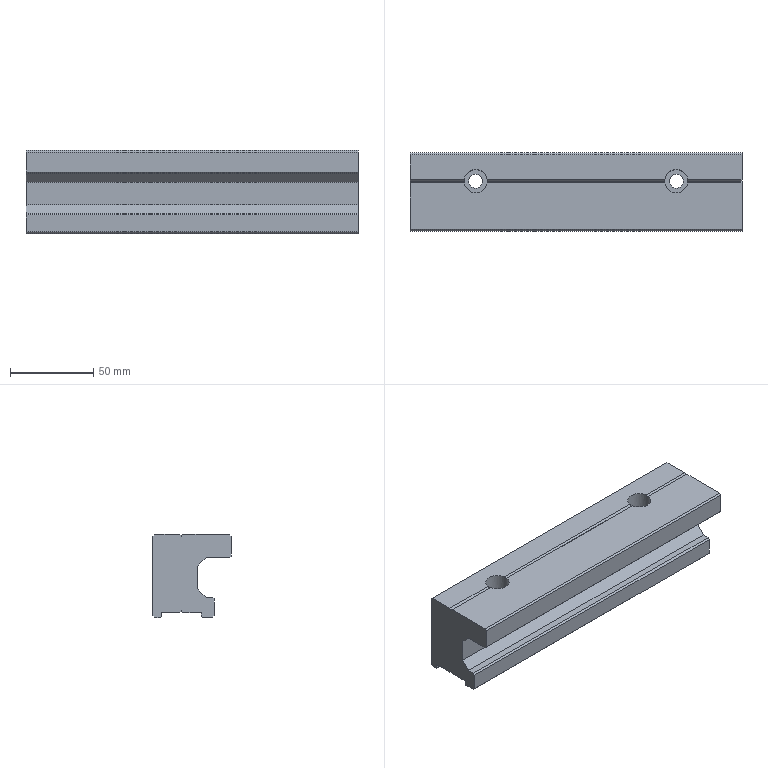Part | NX | features EXTRUDE 3, DATUM_CSYS 2, SKETCH 1 | 1 solid | 44 faces | box 200 x 47 x 50 mm | volume 331921 mm3 | plane 40 | cylinder 4 | commonest cylinder face diameters 8.5 x2 14 x2
STEP:
#1=CARTESIAN_POINT('',(5499.076,6787.516,0.));
#2=VERTEX_POINT('',#1);
#3=CARTESIAN_POINT('',(5485.22,6787.516,0.));
#4=VERTEX_POINT('',#3);
#5=CARTESIAN_POINT('',(5492.148,6786.516,0.));
#6=DIRECTION('',(0.,0.,1.));
#7=DIRECTION('',(1.,0.,0.));
#8=AXIS2_PLACEMENT_3D('',#5,#6,#7);
#9=CIRCLE('',#8,7.);
#10=EDGE_CURVE('',#2,#4,#9,.T.);
#11=ORIENTED_EDGE('',*,*,#10,.F.);
#12=CARTESIAN_POINT('',(5531.718,6787.516,0.));
#13=VERTEX_POINT('',#12);
#14=CARTESIAN_POINT('',(5331.718,6787.516,0.));
#15=DIRECTION('',(1.,0.,0.));
#16=VECTOR('',#15,1000.);
#17=LINE('',#14,#16);
#18=EDGE_CURVE('',#2,#13,#17,.T.);
#19=ORIENTED_EDGE('',*,*,#18,.T.);
#20=CARTESIAN_POINT('',(5531.718,6802.516,0.));
#21=VERTEX_POINT('',#20);
#22=CARTESIAN_POINT('',(5531.718,6787.516,0.));
#23=DIRECTION('',(0.,1.,0.));
#24=VECTOR('',#23,1000.);
#25=LINE('',#22,#24);
#26=EDGE_CURVE('',#13,#21,#25,.T.);
#27=ORIENTED_EDGE('',*,*,#26,.T.);
#28=CARTESIAN_POINT('',(5331.718,6802.516,0.));
#29=VERTEX_POINT('',#28);
#30=CARTESIAN_POINT('',(5331.718,6802.516,0.));
#31=DIRECTION('',(1.,0.,0.));
#32=VECTOR('',#31,1000.);
#33=LINE('',#30,#32);
#34=EDGE_CURVE('',#29,#21,#33,.T.);
#35=ORIENTED_EDGE('',*,*,#34,.F.);
#36=CARTESIAN_POINT('',(5331.718,6787.516,0.));
#37=VERTEX_POINT('',#36);
#38=CARTESIAN_POINT('',(5331.718,6787.516,0.));
#39=DIRECTION('',(0.,1.,0.));
#40=VECTOR('',#39,1000.);
#41=LINE('',#38,#40);
#42=EDGE_CURVE('',#37,#29,#41,.T.);
#43=ORIENTED_EDGE('',*,*,#42,.F.);
#44=CARTESIAN_POINT('',(5364.361,6787.516,0.));
#45=VERTEX_POINT('',#44);
#46=CARTESIAN_POINT('',(5331.718,6787.516,0.));
#47=DIRECTION('',(1.,0.,0.));
#48=VECTOR('',#47,1000.);
#49=LINE('',#46,#48);
#50=EDGE_CURVE('',#37,#45,#49,.T.);
#51=ORIENTED_EDGE('',*,*,#50,.T.);
#52=CARTESIAN_POINT('',(5378.217,6787.516,0.));
#53=VERTEX_POINT('',#52);
#54=CARTESIAN_POINT('',(5371.289,6786.516,0.));
#55=DIRECTION('',(0.,0.,1.));
#56=DIRECTION('',(1.,0.,0.));
#57=AXIS2_PLACEMENT_3D('',#54,#55,#56);
#58=CIRCLE('',#57,7.);
#59=EDGE_CURVE('',#53,#45,#58,.T.);
#60=ORIENTED_EDGE('',*,*,#59,.F.);
#61=CARTESIAN_POINT('',(5331.718,6787.516,0.));
#62=DIRECTION('',(1.,0.,0.));
#63=VECTOR('',#62,1000.);
#64=LINE('',#61,#63);
#65=EDGE_CURVE('',#53,#4,#64,.T.);
#66=ORIENTED_EDGE('',*,*,#65,.T.);
#67=EDGE_LOOP('',(#11,#19,#27,#35,#43,#51,#60,#66));
#68=FACE_BOUND('',#67,.T.);
#69=CARTESIAN_POINT('',(5331.718,6787.516,0.));
#70=DIRECTION('',(0.,0.,-1.));
#71=DIRECTION('',(-1.,0.,0.));
#72=AXIS2_PLACEMENT_3D('',#69,#70,#71);
#73=PLANE('',#72);
#74=ADVANCED_FACE('',(#68),#73,.F.);
#75=CARTESIAN_POINT('',(5485.22,6785.516,0.));
#76=VERTEX_POINT('',#75);
#77=CARTESIAN_POINT('',(5499.076,6785.516,0.));
#78=VERTEX_POINT('',#77);
#79=CARTESIAN_POINT('',(5492.148,6786.516,0.));
#80=DIRECTION('',(0.,0.,1.));
#81=DIRECTION('',(1.,0.,0.));
#82=AXIS2_PLACEMENT_3D('',#79,#80,#81);
#83=CIRCLE('',#82,7.);
#84=EDGE_CURVE('',#76,#78,#83,.T.);
#85=ORIENTED_EDGE('',*,*,#84,.F.);
#86=CARTESIAN_POINT('',(5378.217,6785.516,0.));
#87=VERTEX_POINT('',#86);
#88=CARTESIAN_POINT('',(5331.718,6785.516,0.));
#89=DIRECTION('',(1.,0.,0.));
#90=VECTOR('',#89,1000.);
#91=LINE('',#88,#90);
#92=EDGE_CURVE('',#87,#76,#91,.T.);
#93=ORIENTED_EDGE('',*,*,#92,.F.);
#94=CARTESIAN_POINT('',(5364.361,6785.516,0.));
#95=VERTEX_POINT('',#94);
#96=CARTESIAN_POINT('',(5371.289,6786.516,0.));
#97=DIRECTION('',(0.,0.,1.));
#98=DIRECTION('',(1.,0.,0.));
#99=AXIS2_PLACEMENT_3D('',#96,#97,#98);
#100=CIRCLE('',#99,7.);
#101=EDGE_CURVE('',#95,#87,#100,.T.);
#102=ORIENTED_EDGE('',*,*,#101,.F.);
#103=CARTESIAN_POINT('',(5331.718,6785.516,0.));
#104=VERTEX_POINT('',#103);
#105=CARTESIAN_POINT('',(5331.718,6785.516,0.));
#106=DIRECTION('',(1.,0.,0.));
#107=VECTOR('',#106,1000.);
#108=LINE('',#105,#107);
#109=EDGE_CURVE('',#104,#95,#108,.T.);
#110=ORIENTED_EDGE('',*,*,#109,.F.);
#111=CARTESIAN_POINT('',(5331.718,6757.516,0.));
#112=VERTEX_POINT('',#111);
#113=CARTESIAN_POINT('',(5331.718,6757.516,0.));
#114=DIRECTION('',(0.,1.,0.));
#115=VECTOR('',#114,1000.);
#116=LINE('',#113,#115);
#117=EDGE_CURVE('',#112,#104,#116,.T.);
#118=ORIENTED_EDGE('',*,*,#117,.F.);
#119=CARTESIAN_POINT('',(5531.718,6757.516,0.));
#120=VERTEX_POINT('',#119);
#121=CARTESIAN_POINT('',(5331.718,6757.516,0.));
#122=DIRECTION('',(1.,0.,0.));
#123=VECTOR('',#122,1000.);
#124=LINE('',#121,#123);
#125=EDGE_CURVE('',#112,#120,#124,.T.);
#126=ORIENTED_EDGE('',*,*,#125,.T.);
#127=CARTESIAN_POINT('',(5531.718,6785.516,0.));
#128=VERTEX_POINT('',#127);
#129=CARTESIAN_POINT('',(5531.718,6757.516,0.));
#130=DIRECTION('',(0.,1.,0.));
#131=VECTOR('',#130,1000.);
#132=LINE('',#129,#131);
#133=EDGE_CURVE('',#120,#128,#132,.T.);
#134=ORIENTED_EDGE('',*,*,#133,.T.);
#135=CARTESIAN_POINT('',(5331.718,6785.516,0.));
#136=DIRECTION('',(1.,0.,0.));
#137=VECTOR('',#136,1000.);
#138=LINE('',#135,#137);
#139=EDGE_CURVE('',#78,#128,#138,.T.);
#140=ORIENTED_EDGE('',*,*,#139,.F.);
#141=EDGE_LOOP('',(#85,#93,#102,#110,#118,#126,#134,#140));
#142=FACE_BOUND('',#141,.T.);
#143=CARTESIAN_POINT('',(5331.718,6757.516,0.));
#144=DIRECTION('',(0.,0.,-1.));
#145=DIRECTION('',(-1.,0.,0.));
#146=AXIS2_PLACEMENT_3D('',#143,#144,#145);
#147=PLANE('',#146);
#148=ADVANCED_FACE('',(#142),#147,.F.);
#149=CARTESIAN_POINT('',(5375.419,6785.516,-47.));
#150=VERTEX_POINT('',#149);
#151=CARTESIAN_POINT('',(5367.158,6785.516,-47.));
#152=VERTEX_POINT('',#151);
#153=CARTESIAN_POINT('',(5371.289,6786.516,-47.));
#154=DIRECTION('',(0.,0.,1.));
#155=DIRECTION('',(1.,0.,0.));
#156=AXIS2_PLACEMENT_3D('',#153,#154,#155);
#157=CIRCLE('',#156,4.25);
#158=EDGE_CURVE('',#150,#152,#157,.F.);
#159=ORIENTED_EDGE('',*,*,#158,.T.);
#160=CARTESIAN_POINT('',(5367.039,6786.516,-46.));
#161=VERTEX_POINT('',#160);
#162=CARTESIAN_POINT('',(5371.289,6786.516,-46.));
#163=DIRECTION('',(0.,-0.7071,0.7071));
#164=DIRECTION('',(0.,0.7071,0.7071));
#165=AXIS2_PLACEMENT_3D('',#162,#163,#164);
#166=ELLIPSE('',#165,6.01,4.25);
#167=EDGE_CURVE('',#152,#161,#166,.F.);
#168=ORIENTED_EDGE('',*,*,#167,.T.);
#169=CARTESIAN_POINT('',(5367.158,6787.516,-47.));
#170=VERTEX_POINT('',#169);
#171=CARTESIAN_POINT('',(5371.289,6786.516,-46.));
#172=DIRECTION('',(0.,0.7071,0.7071));
#173=DIRECTION('',(0.,-0.7071,0.7071));
#174=AXIS2_PLACEMENT_3D('',#171,#172,#173);
#175=ELLIPSE('',#174,6.01,4.25);
#176=EDGE_CURVE('',#161,#170,#175,.F.);
#177=ORIENTED_EDGE('',*,*,#176,.T.);
#178=CARTESIAN_POINT('',(5375.419,6787.516,-47.));
#179=VERTEX_POINT('',#178);
#180=CARTESIAN_POINT('',(5371.289,6786.516,-47.));
#181=DIRECTION('',(0.,0.,1.));
#182=DIRECTION('',(1.,0.,0.));
#183=AXIS2_PLACEMENT_3D('',#180,#181,#182);
#184=CIRCLE('',#183,4.25);
#185=EDGE_CURVE('',#170,#179,#184,.F.);
#186=ORIENTED_EDGE('',*,*,#185,.T.);
#187=CARTESIAN_POINT('',(5375.539,6786.516,-46.));
#188=VERTEX_POINT('',#187);
#189=CARTESIAN_POINT('',(5371.289,6786.516,-46.));
#190=DIRECTION('',(0.,0.7071,0.7071));
#191=DIRECTION('',(0.,-0.7071,0.7071));
#192=AXIS2_PLACEMENT_3D('',#189,#190,#191);
#193=ELLIPSE('',#192,6.01,4.25);
#194=EDGE_CURVE('',#179,#188,#193,.F.);
#195=ORIENTED_EDGE('',*,*,#194,.T.);
#196=CARTESIAN_POINT('',(5371.289,6786.516,-46.));
#197=DIRECTION('',(0.,-0.7071,0.7071));
#198=DIRECTION('',(0.,0.7071,0.7071));
#199=AXIS2_PLACEMENT_3D('',#196,#197,#198);
#200=ELLIPSE('',#199,6.01,4.25);
#201=EDGE_CURVE('',#188,#150,#200,.F.);
#202=ORIENTED_EDGE('',*,*,#201,.T.);
#203=EDGE_LOOP('',(#159,#168,#177,#186,#195,#202));
#204=FACE_BOUND('',#203,.T.);
#205=CARTESIAN_POINT('',(5375.539,6786.516,-12.));
#206=VERTEX_POINT('',#205);
#207=CARTESIAN_POINT('',(5371.289,6786.516,-12.));
#208=DIRECTION('',(0.,0.,1.));
#209=DIRECTION('',(1.,0.,0.));
#210=AXIS2_PLACEMENT_3D('',#207,#208,#209);
#211=CIRCLE('',#210,4.25);
#212=EDGE_CURVE('',#206,#206,#211,.F.);
#213=ORIENTED_EDGE('',*,*,#212,.F.);
#214=EDGE_LOOP('',(#213));
#215=FACE_BOUND('',#214,.T.);
#216=CARTESIAN_POINT('',(5371.289,6786.516,-55000.));
#217=DIRECTION('',(0.,0.,1.));
#218=DIRECTION('',(1.,0.,0.));
#219=AXIS2_PLACEMENT_3D('',#216,#217,#218);
#220=CYLINDRICAL_SURFACE('',#219,4.25);
#221=ADVANCED_FACE('',(#204,#215),#220,.F.);
#222=CARTESIAN_POINT('',(5496.279,6785.516,-47.));
#223=VERTEX_POINT('',#222);
#224=CARTESIAN_POINT('',(5488.017,6785.516,-47.));
#225=VERTEX_POINT('',#224);
#226=CARTESIAN_POINT('',(5492.148,6786.516,-47.));
#227=DIRECTION('',(0.,0.,1.));
#228=DIRECTION('',(1.,0.,0.));
#229=AXIS2_PLACEMENT_3D('',#226,#227,#228);
#230=CIRCLE('',#229,4.25);
#231=EDGE_CURVE('',#223,#225,#230,.F.);
#232=ORIENTED_EDGE('',*,*,#231,.T.);
#233=CARTESIAN_POINT('',(5487.898,6786.516,-46.));
#234=VERTEX_POINT('',#233);
#235=CARTESIAN_POINT('',(5492.148,6786.516,-46.));
#236=DIRECTION('',(0.,-0.7071,0.7071));
#237=DIRECTION('',(0.,0.7071,0.7071));
#238=AXIS2_PLACEMENT_3D('',#235,#236,#237);
#239=ELLIPSE('',#238,6.01,4.25);
#240=EDGE_CURVE('',#225,#234,#239,.F.);
#241=ORIENTED_EDGE('',*,*,#240,.T.);
#242=CARTESIAN_POINT('',(5488.017,6787.516,-47.));
#243=VERTEX_POINT('',#242);
#244=CARTESIAN_POINT('',(5492.148,6786.516,-46.));
#245=DIRECTION('',(0.,0.7071,0.7071));
#246=DIRECTION('',(0.,-0.7071,0.7071));
#247=AXIS2_PLACEMENT_3D('',#244,#245,#246);
#248=ELLIPSE('',#247,6.01,4.25);
#249=EDGE_CURVE('',#234,#243,#248,.F.);
#250=ORIENTED_EDGE('',*,*,#249,.T.);
#251=CARTESIAN_POINT('',(5496.279,6787.516,-47.));
#252=VERTEX_POINT('',#251);
#253=CARTESIAN_POINT('',(5492.148,6786.516,-47.));
#254=DIRECTION('',(0.,0.,1.));
#255=DIRECTION('',(1.,0.,0.));
#256=AXIS2_PLACEMENT_3D('',#253,#254,#255);
#257=CIRCLE('',#256,4.25);
#258=EDGE_CURVE('',#243,#252,#257,.F.);
#259=ORIENTED_EDGE('',*,*,#258,.T.);
#260=CARTESIAN_POINT('',(5496.398,6786.516,-46.));
#261=VERTEX_POINT('',#260);
#262=CARTESIAN_POINT('',(5492.148,6786.516,-46.));
#263=DIRECTION('',(0.,0.7071,0.7071));
#264=DIRECTION('',(0.,-0.7071,0.7071));
#265=AXIS2_PLACEMENT_3D('',#262,#263,#264);
#266=ELLIPSE('',#265,6.01,4.25);
#267=EDGE_CURVE('',#252,#261,#266,.F.);
#268=ORIENTED_EDGE('',*,*,#267,.T.);
#269=CARTESIAN_POINT('',(5492.148,6786.516,-46.));
#270=DIRECTION('',(0.,-0.7071,0.7071));
#271=DIRECTION('',(0.,0.7071,0.7071));
#272=AXIS2_PLACEMENT_3D('',#269,#270,#271);
#273=ELLIPSE('',#272,6.01,4.25);
#274=EDGE_CURVE('',#261,#223,#273,.F.);
#275=ORIENTED_EDGE('',*,*,#274,.T.);
#276=EDGE_LOOP('',(#232,#241,#250,#259,#268,#275));
#277=FACE_BOUND('',#276,.T.);
#278=CARTESIAN_POINT('',(5496.398,6786.516,-12.));
#279=VERTEX_POINT('',#278);
#280=CARTESIAN_POINT('',(5492.148,6786.516,-12.));
#281=DIRECTION('',(0.,0.,1.));
#282=DIRECTION('',(1.,0.,0.));
#283=AXIS2_PLACEMENT_3D('',#280,#281,#282);
#284=CIRCLE('',#283,4.25);
#285=EDGE_CURVE('',#279,#279,#284,.F.);
#286=ORIENTED_EDGE('',*,*,#285,.F.);
#287=EDGE_LOOP('',(#286));
#288=FACE_BOUND('',#287,.T.);
#289=CARTESIAN_POINT('',(5492.148,6786.516,-55000.));
#290=DIRECTION('',(0.,0.,1.));
#291=DIRECTION('',(1.,0.,0.));
#292=AXIS2_PLACEMENT_3D('',#289,#290,#291);
#293=CYLINDRICAL_SURFACE('',#292,4.25);
#294=ADVANCED_FACE('',(#277,#288),#293,.F.);
#295=ORIENTED_EDGE('',*,*,#258,.F.);
#296=CARTESIAN_POINT('',(5331.718,6787.516,-47.));
#297=DIRECTION('',(1.,0.,0.));
#298=VECTOR('',#297,1000.);
#299=LINE('',#296,#298);
#300=EDGE_CURVE('',#179,#243,#299,.T.);
#301=ORIENTED_EDGE('',*,*,#300,.F.);
#302=ORIENTED_EDGE('',*,*,#185,.F.);
#303=CARTESIAN_POINT('',(5331.718,6787.516,-47.));
#304=VERTEX_POINT('',#303);
#305=CARTESIAN_POINT('',(5331.718,6787.516,-47.));
#306=DIRECTION('',(1.,0.,0.));
#307=VECTOR('',#306,1000.);
#308=LINE('',#305,#307);
#309=EDGE_CURVE('',#304,#170,#308,.T.);
#310=ORIENTED_EDGE('',*,*,#309,.F.);
#311=CARTESIAN_POINT('',(5331.718,6798.591,-47.));
#312=VERTEX_POINT('',#311);
#313=CARTESIAN_POINT('',(5331.718,6798.591,-47.));
#314=DIRECTION('',(0.,-1.,0.));
#315=VECTOR('',#314,1000.);
#316=LINE('',#313,#315);
#317=EDGE_CURVE('',#312,#304,#316,.T.);
#318=ORIENTED_EDGE('',*,*,#317,.F.);
#319=CARTESIAN_POINT('',(5531.718,6798.591,-47.));
#320=VERTEX_POINT('',#319);
#321=CARTESIAN_POINT('',(5331.718,6798.591,-47.));
#322=DIRECTION('',(1.,0.,0.));
#323=VECTOR('',#322,1000.);
#324=LINE('',#321,#323);
#325=EDGE_CURVE('',#312,#320,#324,.T.);
#326=ORIENTED_EDGE('',*,*,#325,.T.);
#327=CARTESIAN_POINT('',(5531.718,6787.516,-47.));
#328=VERTEX_POINT('',#327);
#329=CARTESIAN_POINT('',(5531.718,6798.591,-47.));
#330=DIRECTION('',(0.,-1.,0.));
#331=VECTOR('',#330,1000.);
#332=LINE('',#329,#331);
#333=EDGE_CURVE('',#320,#328,#332,.T.);
#334=ORIENTED_EDGE('',*,*,#333,.T.);
#335=CARTESIAN_POINT('',(5331.718,6787.516,-47.));
#336=DIRECTION('',(1.,0.,0.));
#337=VECTOR('',#336,1000.);
#338=LINE('',#335,#337);
#339=EDGE_CURVE('',#252,#328,#338,.T.);
#340=ORIENTED_EDGE('',*,*,#339,.F.);
#341=EDGE_LOOP('',(#295,#301,#302,#310,#318,#326,#334,#340));
#342=FACE_BOUND('',#341,.T.);
#343=CARTESIAN_POINT('',(5331.718,6798.591,-47.));
#344=DIRECTION('',(0.,0.,1.));
#345=DIRECTION('',(1.,0.,0.));
#346=AXIS2_PLACEMENT_3D('',#343,#344,#345);
#347=PLANE('',#346);
#348=ADVANCED_FACE('',(#342),#347,.F.);
#349=ORIENTED_EDGE('',*,*,#249,.F.);
#350=CARTESIAN_POINT('',(5331.718,6786.516,-46.));
#351=DIRECTION('',(1.,0.,0.));
#352=VECTOR('',#351,1000.);
#353=LINE('',#350,#352);
#354=EDGE_CURVE('',#188,#234,#353,.T.);
#355=ORIENTED_EDGE('',*,*,#354,.F.);
#356=ORIENTED_EDGE('',*,*,#194,.F.);
#357=ORIENTED_EDGE('',*,*,#300,.T.);
#358=EDGE_LOOP('',(#349,#355,#356,#357));
#359=FACE_BOUND('',#358,.T.);
#360=CARTESIAN_POINT('',(5331.718,6787.516,-47.));
#361=DIRECTION('',(0.,0.7071,0.7071));
#362=DIRECTION('',(0.,-0.7071,0.7071));
#363=AXIS2_PLACEMENT_3D('',#360,#361,#362);
#364=PLANE('',#363);
#365=ADVANCED_FACE('',(#359),#364,.F.);
#366=ORIENTED_EDGE('',*,*,#267,.F.);
#367=ORIENTED_EDGE('',*,*,#339,.T.);
#368=CARTESIAN_POINT('',(5531.718,6786.516,-46.));
#369=VERTEX_POINT('',#368);
#370=CARTESIAN_POINT('',(5531.718,6787.516,-47.));
#371=DIRECTION('',(0.,-0.7071,0.7071));
#372=VECTOR('',#371,1000.);
#373=LINE('',#370,#372);
#374=EDGE_CURVE('',#328,#369,#373,.T.);
#375=ORIENTED_EDGE('',*,*,#374,.T.);
#376=CARTESIAN_POINT('',(5331.718,6786.516,-46.));
#377=DIRECTION('',(1.,0.,0.));
#378=VECTOR('',#377,1000.);
#379=LINE('',#376,#378);
#380=EDGE_CURVE('',#261,#369,#379,.T.);
#381=ORIENTED_EDGE('',*,*,#380,.F.);
#382=EDGE_LOOP('',(#366,#367,#375,#381));
#383=FACE_BOUND('',#382,.T.);
#384=CARTESIAN_POINT('',(5331.718,6787.516,-47.));
#385=DIRECTION('',(0.,0.7071,0.7071));
#386=DIRECTION('',(0.,-0.7071,0.7071));
#387=AXIS2_PLACEMENT_3D('',#384,#385,#386);
#388=PLANE('',#387);
#389=ADVANCED_FACE('',(#383),#388,.F.);
#390=ORIENTED_EDGE('',*,*,#176,.F.);
#391=CARTESIAN_POINT('',(5331.718,6786.516,-46.));
#392=VERTEX_POINT('',#391);
#393=CARTESIAN_POINT('',(5331.718,6786.516,-46.));
#394=DIRECTION('',(1.,0.,0.));
#395=VECTOR('',#394,1000.);
#396=LINE('',#393,#395);
#397=EDGE_CURVE('',#392,#161,#396,.T.);
#398=ORIENTED_EDGE('',*,*,#397,.F.);
#399=CARTESIAN_POINT('',(5331.718,6787.516,-47.));
#400=DIRECTION('',(0.,-0.7071,0.7071));
#401=VECTOR('',#400,1000.);
#402=LINE('',#399,#401);
#403=EDGE_CURVE('',#304,#392,#402,.T.);
#404=ORIENTED_EDGE('',*,*,#403,.F.);
#405=ORIENTED_EDGE('',*,*,#309,.T.);
#406=EDGE_LOOP('',(#390,#398,#404,#405));
#407=FACE_BOUND('',#406,.T.);
#408=CARTESIAN_POINT('',(5331.718,6787.516,-47.));
#409=DIRECTION('',(0.,0.7071,0.7071));
#410=DIRECTION('',(0.,-0.7071,0.7071));
#411=AXIS2_PLACEMENT_3D('',#408,#409,#410);
#412=PLANE('',#411);
#413=ADVANCED_FACE('',(#407),#412,.F.);
#414=ORIENTED_EDGE('',*,*,#274,.F.);
#415=ORIENTED_EDGE('',*,*,#380,.T.);
#416=CARTESIAN_POINT('',(5531.718,6785.516,-47.));
#417=VERTEX_POINT('',#416);
#418=CARTESIAN_POINT('',(5531.718,6786.516,-46.));
#419=DIRECTION('',(0.,-0.7071,-0.7071));
#420=VECTOR('',#419,1000.);
#421=LINE('',#418,#420);
#422=EDGE_CURVE('',#369,#417,#421,.T.);
#423=ORIENTED_EDGE('',*,*,#422,.T.);
#424=CARTESIAN_POINT('',(5331.718,6785.516,-47.));
#425=DIRECTION('',(1.,0.,0.));
#426=VECTOR('',#425,1000.);
#427=LINE('',#424,#426);
#428=EDGE_CURVE('',#223,#417,#427,.T.);
#429=ORIENTED_EDGE('',*,*,#428,.F.);
#430=EDGE_LOOP('',(#414,#415,#423,#429));
#431=FACE_BOUND('',#430,.T.);
#432=CARTESIAN_POINT('',(5331.718,6786.516,-46.));
#433=DIRECTION('',(0.,-0.7071,0.7071));
#434=DIRECTION('',(0.,-0.7071,-0.7071));
#435=AXIS2_PLACEMENT_3D('',#432,#433,#434);
#436=PLANE('',#435);
#437=ADVANCED_FACE('',(#431),#436,.F.);
#438=ORIENTED_EDGE('',*,*,#240,.F.);
#439=CARTESIAN_POINT('',(5331.718,6785.516,-47.));
#440=DIRECTION('',(1.,0.,0.));
#441=VECTOR('',#440,1000.);
#442=LINE('',#439,#441);
#443=EDGE_CURVE('',#150,#225,#442,.T.);
#444=ORIENTED_EDGE('',*,*,#443,.F.);
#445=ORIENTED_EDGE('',*,*,#201,.F.);
#446=ORIENTED_EDGE('',*,*,#354,.T.);
#447=EDGE_LOOP('',(#438,#444,#445,#446));
#448=FACE_BOUND('',#447,.T.);
#449=CARTESIAN_POINT('',(5331.718,6786.516,-46.));
#450=DIRECTION('',(0.,-0.7071,0.7071));
#451=DIRECTION('',(0.,-0.7071,-0.7071));
#452=AXIS2_PLACEMENT_3D('',#449,#450,#451);
#453=PLANE('',#452);
#454=ADVANCED_FACE('',(#448),#453,.F.);
#455=ORIENTED_EDGE('',*,*,#167,.F.);
#456=CARTESIAN_POINT('',(5331.718,6785.516,-47.));
#457=VERTEX_POINT('',#456);
#458=CARTESIAN_POINT('',(5331.718,6785.516,-47.));
#459=DIRECTION('',(1.,0.,0.));
#460=VECTOR('',#459,1000.);
#461=LINE('',#458,#460);
#462=EDGE_CURVE('',#457,#152,#461,.T.);
#463=ORIENTED_EDGE('',*,*,#462,.F.);
#464=CARTESIAN_POINT('',(5331.718,6786.516,-46.));
#465=DIRECTION('',(0.,-0.7071,-0.7071));
#466=VECTOR('',#465,1000.);
#467=LINE('',#464,#466);
#468=EDGE_CURVE('',#392,#457,#467,.T.);
#469=ORIENTED_EDGE('',*,*,#468,.F.);
#470=ORIENTED_EDGE('',*,*,#397,.T.);
#471=EDGE_LOOP('',(#455,#463,#469,#470));
#472=FACE_BOUND('',#471,.T.);
#473=CARTESIAN_POINT('',(5331.718,6786.516,-46.));
#474=DIRECTION('',(0.,-0.7071,0.7071));
#475=DIRECTION('',(0.,-0.7071,-0.7071));
#476=AXIS2_PLACEMENT_3D('',#473,#474,#475);
#477=PLANE('',#476);
#478=ADVANCED_FACE('',(#472),#477,.F.);
#479=ORIENTED_EDGE('',*,*,#231,.F.);
#480=ORIENTED_EDGE('',*,*,#428,.T.);
#481=CARTESIAN_POINT('',(5531.718,6774.441,-47.));
#482=VERTEX_POINT('',#481);
#483=CARTESIAN_POINT('',(5531.718,6785.516,-47.));
#484=DIRECTION('',(0.,-1.,0.));
#485=VECTOR('',#484,1000.);
#486=LINE('',#483,#485);
#487=EDGE_CURVE('',#417,#482,#486,.T.);
#488=ORIENTED_EDGE('',*,*,#487,.T.);
#489=CARTESIAN_POINT('',(5331.718,6774.441,-47.));
#490=VERTEX_POINT('',#489);
#491=CARTESIAN_POINT('',(5331.718,6774.441,-47.));
#492=DIRECTION('',(1.,0.,0.));
#493=VECTOR('',#492,1000.);
#494=LINE('',#491,#493);
#495=EDGE_CURVE('',#490,#482,#494,.T.);
#496=ORIENTED_EDGE('',*,*,#495,.F.);
#497=CARTESIAN_POINT('',(5331.718,6785.516,-47.));
#498=DIRECTION('',(0.,-1.,0.));
#499=VECTOR('',#498,1000.);
#500=LINE('',#497,#499);
#501=EDGE_CURVE('',#457,#490,#500,.T.);
#502=ORIENTED_EDGE('',*,*,#501,.F.);
#503=ORIENTED_EDGE('',*,*,#462,.T.);
#504=ORIENTED_EDGE('',*,*,#158,.F.);
#505=ORIENTED_EDGE('',*,*,#443,.T.);
#506=EDGE_LOOP('',(#479,#480,#488,#496,#502,#503,#504,#505));
#507=FACE_BOUND('',#506,.T.);
#508=CARTESIAN_POINT('',(5331.718,6785.516,-47.));
#509=DIRECTION('',(0.,0.,1.));
#510=DIRECTION('',(1.,0.,0.));
#511=AXIS2_PLACEMENT_3D('',#508,#509,#510);
#512=PLANE('',#511);
#513=ADVANCED_FACE('',(#507),#512,.F.);
#514=ORIENTED_EDGE('',*,*,#92,.T.);
#515=CARTESIAN_POINT('',(5485.148,6786.516,-1.));
#516=VERTEX_POINT('',#515);
#517=CARTESIAN_POINT('',(5492.148,6786.516,-1.));
#518=DIRECTION('',(0.,-0.7071,-0.7071));
#519=DIRECTION('',(0.,-0.7071,0.7071));
#520=AXIS2_PLACEMENT_3D('',#517,#518,#519);
#521=ELLIPSE('',#520,9.899,7.);
#522=EDGE_CURVE('',#76,#516,#521,.T.);
#523=ORIENTED_EDGE('',*,*,#522,.T.);
#524=CARTESIAN_POINT('',(5378.289,6786.516,-1.));
#525=VERTEX_POINT('',#524);
#526=CARTESIAN_POINT('',(5331.718,6786.516,-1.));
#527=DIRECTION('',(1.,0.,0.));
#528=VECTOR('',#527,1000.);
#529=LINE('',#526,#528);
#530=EDGE_CURVE('',#525,#516,#529,.T.);
#531=ORIENTED_EDGE('',*,*,#530,.F.);
#532=CARTESIAN_POINT('',(5371.289,6786.516,-1.));
#533=DIRECTION('',(0.,-0.7071,-0.7071));
#534=DIRECTION('',(0.,-0.7071,0.7071));
#535=AXIS2_PLACEMENT_3D('',#532,#533,#534);
#536=ELLIPSE('',#535,9.899,7.);
#537=EDGE_CURVE('',#525,#87,#536,.T.);
#538=ORIENTED_EDGE('',*,*,#537,.T.);
#539=EDGE_LOOP('',(#514,#523,#531,#538));
#540=FACE_BOUND('',#539,.T.);
#541=CARTESIAN_POINT('',(5331.718,6785.516,0.));
#542=DIRECTION('',(0.,-0.7071,-0.7071));
#543=DIRECTION('',(0.,0.7071,-0.7071));
#544=AXIS2_PLACEMENT_3D('',#541,#542,#543);
#545=PLANE('',#544);
#546=ADVANCED_FACE('',(#540),#545,.F.);
#547=ORIENTED_EDGE('',*,*,#109,.T.);
#548=CARTESIAN_POINT('',(5364.289,6786.516,-1.));
#549=VERTEX_POINT('',#548);
#550=CARTESIAN_POINT('',(5371.289,6786.516,-1.));
#551=DIRECTION('',(0.,-0.7071,-0.7071));
#552=DIRECTION('',(0.,-0.7071,0.7071));
#553=AXIS2_PLACEMENT_3D('',#550,#551,#552);
#554=ELLIPSE('',#553,9.899,7.);
#555=EDGE_CURVE('',#95,#549,#554,.T.);
#556=ORIENTED_EDGE('',*,*,#555,.T.);
#557=CARTESIAN_POINT('',(5331.718,6786.516,-1.));
#558=VERTEX_POINT('',#557);
#559=CARTESIAN_POINT('',(5331.718,6786.516,-1.));
#560=DIRECTION('',(1.,0.,0.));
#561=VECTOR('',#560,1000.);
#562=LINE('',#559,#561);
#563=EDGE_CURVE('',#558,#549,#562,.T.);
#564=ORIENTED_EDGE('',*,*,#563,.F.);
#565=CARTESIAN_POINT('',(5331.718,6785.516,0.));
#566=DIRECTION('',(0.,0.7071,-0.7071));
#567=VECTOR('',#566,1000.);
#568=LINE('',#565,#567);
#569=EDGE_CURVE('',#104,#558,#568,.T.);
#570=ORIENTED_EDGE('',*,*,#569,.F.);
#571=EDGE_LOOP('',(#547,#556,#564,#570));
#572=FACE_BOUND('',#571,.T.);
#573=CARTESIAN_POINT('',(5331.718,6785.516,0.));
#574=DIRECTION('',(0.,-0.7071,-0.7071));
#575=DIRECTION('',(0.,0.7071,-0.7071));
#576=AXIS2_PLACEMENT_3D('',#573,#574,#575);
#577=PLANE('',#576);
#578=ADVANCED_FACE('',(#572),#577,.F.);
#579=ORIENTED_EDGE('',*,*,#18,.F.);
#580=CARTESIAN_POINT('',(5499.148,6786.516,-1.));
#581=VERTEX_POINT('',#580);
#582=CARTESIAN_POINT('',(5492.148,6786.516,-1.));
#583=DIRECTION('',(0.,0.7071,-0.7071));
#584=DIRECTION('',(0.,0.7071,0.7071));
#585=AXIS2_PLACEMENT_3D('',#582,#583,#584);
#586=ELLIPSE('',#585,9.899,7.);
#587=EDGE_CURVE('',#2,#581,#586,.T.);
#588=ORIENTED_EDGE('',*,*,#587,.T.);
#589=CARTESIAN_POINT('',(5531.718,6786.516,-1.));
#590=VERTEX_POINT('',#589);
#591=CARTESIAN_POINT('',(5331.718,6786.516,-1.));
#592=DIRECTION('',(1.,0.,0.));
#593=VECTOR('',#592,1000.);
#594=LINE('',#591,#593);
#595=EDGE_CURVE('',#581,#590,#594,.T.);
#596=ORIENTED_EDGE('',*,*,#595,.T.);
#597=CARTESIAN_POINT('',(5531.718,6786.516,-1.));
#598=DIRECTION('',(0.,0.7071,0.7071));
#599=VECTOR('',#598,1000.);
#600=LINE('',#597,#599);
#601=EDGE_CURVE('',#590,#13,#600,.T.);
#602=ORIENTED_EDGE('',*,*,#601,.T.);
#603=EDGE_LOOP('',(#579,#588,#596,#602));
#604=FACE_BOUND('',#603,.T.);
#605=CARTESIAN_POINT('',(5331.718,6786.516,-1.));
#606=DIRECTION('',(0.,0.7071,-0.7071));
#607=DIRECTION('',(0.,0.7071,0.7071));
#608=AXIS2_PLACEMENT_3D('',#605,#606,#607);
#609=PLANE('',#608);
#610=ADVANCED_FACE('',(#604),#609,.F.);
#611=ORIENTED_EDGE('',*,*,#530,.T.);
#612=CARTESIAN_POINT('',(5492.148,6786.516,-1.));
#613=DIRECTION('',(0.,0.7071,-0.7071));
#614=DIRECTION('',(0.,0.7071,0.7071));
#615=AXIS2_PLACEMENT_3D('',#612,#613,#614);
#616=ELLIPSE('',#615,9.899,7.);
#617=EDGE_CURVE('',#516,#4,#616,.T.);
#618=ORIENTED_EDGE('',*,*,#617,.T.);
#619=ORIENTED_EDGE('',*,*,#65,.F.);
#620=CARTESIAN_POINT('',(5371.289,6786.516,-1.));
#621=DIRECTION('',(0.,0.7071,-0.7071));
#622=DIRECTION('',(0.,0.7071,0.7071));
#623=AXIS2_PLACEMENT_3D('',#620,#621,#622);
#624=ELLIPSE('',#623,9.899,7.);
#625=EDGE_CURVE('',#53,#525,#624,.T.);
#626=ORIENTED_EDGE('',*,*,#625,.T.);
#627=EDGE_LOOP('',(#611,#618,#619,#626));
#628=FACE_BOUND('',#627,.T.);
#629=CARTESIAN_POINT('',(5331.718,6786.516,-1.));
#630=DIRECTION('',(0.,0.7071,-0.7071));
#631=DIRECTION('',(0.,0.7071,0.7071));
#632=AXIS2_PLACEMENT_3D('',#629,#630,#631);
#633=PLANE('',#632);
#634=ADVANCED_FACE('',(#628),#633,.F.);
#635=CARTESIAN_POINT('',(5531.718,6803.516,-1.));
#636=VERTEX_POINT('',#635);
#637=CARTESIAN_POINT('',(5531.718,6802.516,0.));
#638=DIRECTION('',(0.,0.7071,-0.7071));
#639=VECTOR('',#638,1000.);
#640=LINE('',#637,#639);
#641=EDGE_CURVE('',#21,#636,#640,.T.);
#642=ORIENTED_EDGE('',*,*,#641,.T.);
#643=CARTESIAN_POINT('',(5331.718,6803.516,-1.));
#644=VERTEX_POINT('',#643);
#645=CARTESIAN_POINT('',(5331.718,6803.516,-1.));
#646=DIRECTION('',(1.,0.,0.));
#647=VECTOR('',#646,1000.);
#648=LINE('',#645,#647);
#649=EDGE_CURVE('',#644,#636,#648,.T.);
#650=ORIENTED_EDGE('',*,*,#649,.F.);
#651=CARTESIAN_POINT('',(5331.718,6802.516,0.));
#652=DIRECTION('',(0.,0.7071,-0.7071));
#653=VECTOR('',#652,1000.);
#654=LINE('',#651,#653);
#655=EDGE_CURVE('',#29,#644,#654,.T.);
#656=ORIENTED_EDGE('',*,*,#655,.F.);
#657=ORIENTED_EDGE('',*,*,#34,.T.);
#658=EDGE_LOOP('',(#642,#650,#656,#657));
#659=FACE_BOUND('',#658,.T.);
#660=CARTESIAN_POINT('',(5331.718,6802.516,0.));
#661=DIRECTION('',(0.,-0.7071,-0.7071));
#662=DIRECTION('',(0.,0.7071,-0.7071));
#663=AXIS2_PLACEMENT_3D('',#660,#661,#662);
#664=PLANE('',#663);
#665=ADVANCED_FACE('',(#659),#664,.F.);
#666=CARTESIAN_POINT('',(5531.718,6803.516,-49.));
#667=VERTEX_POINT('',#666);
#668=CARTESIAN_POINT('',(5531.718,6803.516,-1.));
#669=DIRECTION('',(0.,0.,-1.));
#670=VECTOR('',#669,1000.);
#671=LINE('',#668,#670);
#672=EDGE_CURVE('',#636,#667,#671,.T.);
#673=ORIENTED_EDGE('',*,*,#672,.T.);
#674=CARTESIAN_POINT('',(5331.718,6803.516,-49.));
#675=VERTEX_POINT('',#674);
#676=CARTESIAN_POINT('',(5331.718,6803.516,-49.));
#677=DIRECTION('',(1.,0.,0.));
#678=VECTOR('',#677,1000.);
#679=LINE('',#676,#678);
#680=EDGE_CURVE('',#675,#667,#679,.T.);
#681=ORIENTED_EDGE('',*,*,#680,.F.);
#682=CARTESIAN_POINT('',(5331.718,6803.516,-1.));
#683=DIRECTION('',(0.,0.,-1.));
#684=VECTOR('',#683,1000.);
#685=LINE('',#682,#684);
#686=EDGE_CURVE('',#644,#675,#685,.T.);
#687=ORIENTED_EDGE('',*,*,#686,.F.);
#688=ORIENTED_EDGE('',*,*,#649,.T.);
#689=EDGE_LOOP('',(#673,#681,#687,#688));
#690=FACE_BOUND('',#689,.T.);
#691=CARTESIAN_POINT('',(5331.718,6803.516,-1.));
#692=DIRECTION('',(0.,-1.,0.));
#693=DIRECTION('',(0.,0.,-1.));
#694=AXIS2_PLACEMENT_3D('',#691,#692,#693);
#695=PLANE('',#694);
#696=ADVANCED_FACE('',(#690),#695,.F.);
#697=CARTESIAN_POINT('',(5531.718,6802.516,-50.));
#698=VERTEX_POINT('',#697);
#699=CARTESIAN_POINT('',(5531.718,6803.516,-49.));
#700=DIRECTION('',(0.,-0.7071,-0.7071));
#701=VECTOR('',#700,1000.);
#702=LINE('',#699,#701);
#703=EDGE_CURVE('',#667,#698,#702,.T.);
#704=ORIENTED_EDGE('',*,*,#703,.T.);
#705=CARTESIAN_POINT('',(5331.718,6802.516,-50.));
#706=VERTEX_POINT('',#705);
#707=CARTESIAN_POINT('',(5331.718,6802.516,-50.));
#708=DIRECTION('',(1.,0.,0.));
#709=VECTOR('',#708,1000.);
#710=LINE('',#707,#709);
#711=EDGE_CURVE('',#706,#698,#710,.T.);
#712=ORIENTED_EDGE('',*,*,#711,.F.);
#713=CARTESIAN_POINT('',(5331.718,6803.516,-49.));
#714=DIRECTION('',(0.,-0.7071,-0.7071));
#715=VECTOR('',#714,1000.);
#716=LINE('',#713,#715);
#717=EDGE_CURVE('',#675,#706,#716,.T.);
#718=ORIENTED_EDGE('',*,*,#717,.F.);
#719=ORIENTED_EDGE('',*,*,#680,.T.);
#720=EDGE_LOOP('',(#704,#712,#718,#719));
#721=FACE_BOUND('',#720,.T.);
#722=CARTESIAN_POINT('',(5331.718,6803.516,-49.));
#723=DIRECTION('',(0.,-0.7071,0.7071));
#724=DIRECTION('',(0.,-0.7071,-0.7071));
#725=AXIS2_PLACEMENT_3D('',#722,#723,#724);
#726=PLANE('',#725);
#727=ADVANCED_FACE('',(#721),#726,.F.);
#728=CARTESIAN_POINT('',(5531.718,6799.091,-50.));
#729=VERTEX_POINT('',#728);
#730=CARTESIAN_POINT('',(5531.718,6802.516,-50.));
#731=DIRECTION('',(0.,-1.,0.));
#732=VECTOR('',#731,1000.);
#733=LINE('',#730,#732);
#734=EDGE_CURVE('',#698,#729,#733,.T.);
#735=ORIENTED_EDGE('',*,*,#734,.T.);
#736=CARTESIAN_POINT('',(5331.718,6799.091,-50.));
#737=VERTEX_POINT('',#736);
#738=CARTESIAN_POINT('',(5331.718,6799.091,-50.));
#739=DIRECTION('',(1.,0.,0.));
#740=VECTOR('',#739,1000.);
#741=LINE('',#738,#740);
#742=EDGE_CURVE('',#737,#729,#741,.T.);
#743=ORIENTED_EDGE('',*,*,#742,.F.);
#744=CARTESIAN_POINT('',(5331.718,6802.516,-50.));
#745=DIRECTION('',(0.,-1.,0.));
#746=VECTOR('',#745,1000.);
#747=LINE('',#744,#746);
#748=EDGE_CURVE('',#706,#737,#747,.T.);
#749=ORIENTED_EDGE('',*,*,#748,.F.);
#750=ORIENTED_EDGE('',*,*,#711,.T.);
#751=EDGE_LOOP('',(#735,#743,#749,#750));
#752=FACE_BOUND('',#751,.T.);
#753=CARTESIAN_POINT('',(5331.718,6802.516,-50.));
#754=DIRECTION('',(0.,0.,1.));
#755=DIRECTION('',(1.,0.,0.));
#756=AXIS2_PLACEMENT_3D('',#753,#754,#755);
#757=PLANE('',#756);
#758=ADVANCED_FACE('',(#752),#757,.F.);
#759=CARTESIAN_POINT('',(5531.718,6798.591,-49.5));
#760=VERTEX_POINT('',#759);
#761=CARTESIAN_POINT('',(5531.718,6799.091,-50.));
#762=DIRECTION('',(0.,-0.7071,0.7071));
#763=VECTOR('',#762,1000.);
#764=LINE('',#761,#763);
#765=EDGE_CURVE('',#729,#760,#764,.T.);
#766=ORIENTED_EDGE('',*,*,#765,.T.);
#767=CARTESIAN_POINT('',(5331.718,6798.591,-49.5));
#768=VERTEX_POINT('',#767);
#769=CARTESIAN_POINT('',(5331.718,6798.591,-49.5));
#770=DIRECTION('',(1.,0.,0.));
#771=VECTOR('',#770,1000.);
#772=LINE('',#769,#771);
#773=EDGE_CURVE('',#768,#760,#772,.T.);
#774=ORIENTED_EDGE('',*,*,#773,.F.);
#775=CARTESIAN_POINT('',(5331.718,6799.091,-50.));
#776=DIRECTION('',(0.,-0.7071,0.7071));
#777=VECTOR('',#776,1000.);
#778=LINE('',#775,#777);
#779=EDGE_CURVE('',#737,#768,#778,.T.);
#780=ORIENTED_EDGE('',*,*,#779,.F.);
#781=ORIENTED_EDGE('',*,*,#742,.T.);
#782=EDGE_LOOP('',(#766,#774,#780,#781));
#783=FACE_BOUND('',#782,.T.);
#784=CARTESIAN_POINT('',(5331.718,6799.091,-50.));
#785=DIRECTION('',(0.,0.7071,0.7071));
#786=DIRECTION('',(0.,-0.7071,0.7071));
#787=AXIS2_PLACEMENT_3D('',#784,#785,#786);
#788=PLANE('',#787);
#789=ADVANCED_FACE('',(#783),#788,.F.);
#790=CARTESIAN_POINT('',(5531.718,6798.591,-49.5));
#791=DIRECTION('',(0.,0.,1.));
#792=VECTOR('',#791,1000.);
#793=LINE('',#790,#792);
#794=EDGE_CURVE('',#760,#320,#793,.T.);
#795=ORIENTED_EDGE('',*,*,#794,.T.);
#796=ORIENTED_EDGE('',*,*,#325,.F.);
#797=CARTESIAN_POINT('',(5331.718,6798.591,-49.5));
#798=DIRECTION('',(0.,0.,1.));
#799=VECTOR('',#798,1000.);
#800=LINE('',#797,#799);
#801=EDGE_CURVE('',#768,#312,#800,.T.);
#802=ORIENTED_EDGE('',*,*,#801,.F.);
#803=ORIENTED_EDGE('',*,*,#773,.T.);
#804=EDGE_LOOP('',(#795,#796,#802,#803));
#805=FACE_BOUND('',#804,.T.);
#806=CARTESIAN_POINT('',(5331.718,6798.591,-49.5));
#807=DIRECTION('',(0.,1.,0.));
#808=DIRECTION('',(0.,0.,1.));
#809=AXIS2_PLACEMENT_3D('',#806,#807,#808);
#810=PLANE('',#809);
#811=ADVANCED_FACE('',(#805),#810,.F.);
#812=CARTESIAN_POINT('',(5531.718,6774.441,-49.3));
#813=VERTEX_POINT('',#812);
#814=CARTESIAN_POINT('',(5531.718,6774.441,-47.));
#815=DIRECTION('',(0.,0.,-1.));
#816=VECTOR('',#815,1000.);
#817=LINE('',#814,#816);
#818=EDGE_CURVE('',#482,#813,#817,.T.);
#819=ORIENTED_EDGE('',*,*,#818,.T.);
#820=CARTESIAN_POINT('',(5331.718,6774.441,-49.3));
#821=VERTEX_POINT('',#820);
#822=CARTESIAN_POINT('',(5331.718,6774.441,-49.3));
#823=DIRECTION('',(1.,0.,0.));
#824=VECTOR('',#823,1000.);
#825=LINE('',#822,#824);
#826=EDGE_CURVE('',#821,#813,#825,.T.);
#827=ORIENTED_EDGE('',*,*,#826,.F.);
#828=CARTESIAN_POINT('',(5331.718,6774.441,-47.));
#829=DIRECTION('',(0.,0.,-1.));
#830=VECTOR('',#829,1000.);
#831=LINE('',#828,#830);
#832=EDGE_CURVE('',#490,#821,#831,.T.);
#833=ORIENTED_EDGE('',*,*,#832,.F.);
#834=ORIENTED_EDGE('',*,*,#495,.T.);
#835=EDGE_LOOP('',(#819,#827,#833,#834));
#836=FACE_BOUND('',#835,.T.);
#837=CARTESIAN_POINT('',(5331.718,6774.441,-47.));
#838=DIRECTION('',(0.,-1.,0.));
#839=DIRECTION('',(0.,0.,-1.));
#840=AXIS2_PLACEMENT_3D('',#837,#838,#839);
#841=PLANE('',#840);
#842=ADVANCED_FACE('',(#836),#841,.F.);
#843=CARTESIAN_POINT('',(5531.718,6773.941,-49.8));
#844=VERTEX_POINT('',#843);
#845=CARTESIAN_POINT('',(5531.718,6774.441,-49.3));
#846=DIRECTION('',(0.,-0.7071,-0.7071));
#847=VECTOR('',#846,1000.);
#848=LINE('',#845,#847);
#849=EDGE_CURVE('',#813,#844,#848,.T.);
#850=ORIENTED_EDGE('',*,*,#849,.T.);
#851=CARTESIAN_POINT('',(5331.718,6773.941,-49.8));
#852=VERTEX_POINT('',#851);
#853=CARTESIAN_POINT('',(5331.718,6773.941,-49.8));
#854=DIRECTION('',(1.,0.,0.));
#855=VECTOR('',#854,1000.);
#856=LINE('',#853,#855);
#857=EDGE_CURVE('',#852,#844,#856,.T.);
#858=ORIENTED_EDGE('',*,*,#857,.F.);
#859=CARTESIAN_POINT('',(5331.718,6774.441,-49.3));
#860=DIRECTION('',(0.,-0.7071,-0.7071));
#861=VECTOR('',#860,1000.);
#862=LINE('',#859,#861);
#863=EDGE_CURVE('',#821,#852,#862,.T.);
#864=ORIENTED_EDGE('',*,*,#863,.F.);
#865=ORIENTED_EDGE('',*,*,#826,.T.);
#866=EDGE_LOOP('',(#850,#858,#864,#865));
#867=FACE_BOUND('',#866,.T.);
#868=CARTESIAN_POINT('',(5331.718,6774.441,-49.3));
#869=DIRECTION('',(0.,-0.7071,0.7071));
#870=DIRECTION('',(0.,-0.7071,-0.7071));
#871=AXIS2_PLACEMENT_3D('',#868,#869,#870);
#872=PLANE('',#871);
#873=ADVANCED_FACE('',(#867),#872,.F.);
#874=CARTESIAN_POINT('',(5531.718,6767.516,-49.8));
#875=VERTEX_POINT('',#874);
#876=CARTESIAN_POINT('',(5531.718,6773.941,-49.8));
#877=DIRECTION('',(0.,-1.,0.));
#878=VECTOR('',#877,1000.);
#879=LINE('',#876,#878);
#880=EDGE_CURVE('',#844,#875,#879,.T.);
#881=ORIENTED_EDGE('',*,*,#880,.T.);
#882=CARTESIAN_POINT('',(5331.718,6767.516,-49.8));
#883=VERTEX_POINT('',#882);
#884=CARTESIAN_POINT('',(5331.718,6767.516,-49.8));
#885=DIRECTION('',(1.,0.,0.));
#886=VECTOR('',#885,1000.);
#887=LINE('',#884,#886);
#888=EDGE_CURVE('',#883,#875,#887,.T.);
#889=ORIENTED_EDGE('',*,*,#888,.F.);
#890=CARTESIAN_POINT('',(5331.718,6773.941,-49.8));
#891=DIRECTION('',(0.,-1.,0.));
#892=VECTOR('',#891,1000.);
#893=LINE('',#890,#892);
#894=EDGE_CURVE('',#852,#883,#893,.T.);
#895=ORIENTED_EDGE('',*,*,#894,.F.);
#896=ORIENTED_EDGE('',*,*,#857,.T.);
#897=EDGE_LOOP('',(#881,#889,#895,#896));
#898=FACE_BOUND('',#897,.T.);
#899=CARTESIAN_POINT('',(5331.718,6773.941,-49.8));
#900=DIRECTION('',(0.,0.,1.));
#901=DIRECTION('',(1.,0.,0.));
#902=AXIS2_PLACEMENT_3D('',#899,#900,#901);
#903=PLANE('',#902);
#904=ADVANCED_FACE('',(#898),#903,.F.);
#905=CARTESIAN_POINT('',(5531.718,6766.516,-48.8));
#906=VERTEX_POINT('',#905);
#907=CARTESIAN_POINT('',(5531.718,6767.516,-49.8));
#908=DIRECTION('',(0.,-0.7071,0.7071));
#909=VECTOR('',#908,1000.);
#910=LINE('',#907,#909);
#911=EDGE_CURVE('',#875,#906,#910,.T.);
#912=ORIENTED_EDGE('',*,*,#911,.T.);
#913=CARTESIAN_POINT('',(5331.718,6766.516,-48.8));
#914=VERTEX_POINT('',#913);
#915=CARTESIAN_POINT('',(5331.718,6766.516,-48.8));
#916=DIRECTION('',(1.,0.,0.));
#917=VECTOR('',#916,1000.);
#918=LINE('',#915,#917);
#919=EDGE_CURVE('',#914,#906,#918,.T.);
#920=ORIENTED_EDGE('',*,*,#919,.F.);
#921=CARTESIAN_POINT('',(5331.718,6767.516,-49.8));
#922=DIRECTION('',(0.,-0.7071,0.7071));
#923=VECTOR('',#922,1000.);
#924=LINE('',#921,#923);
#925=EDGE_CURVE('',#883,#914,#924,.T.);
#926=ORIENTED_EDGE('',*,*,#925,.F.);
#927=ORIENTED_EDGE('',*,*,#888,.T.);
#928=EDGE_LOOP('',(#912,#920,#926,#927));
#929=FACE_BOUND('',#928,.T.);
#930=CARTESIAN_POINT('',(5331.718,6767.516,-49.8));
#931=DIRECTION('',(0.,0.7071,0.7071));
#932=DIRECTION('',(0.,-0.7071,0.7071));
#933=AXIS2_PLACEMENT_3D('',#930,#931,#932);
#934=PLANE('',#933);
#935=ADVANCED_FACE('',(#929),#934,.F.);
#936=CARTESIAN_POINT('',(5531.718,6766.516,-38.8));
#937=VERTEX_POINT('',#936);
#938=CARTESIAN_POINT('',(5531.718,6766.516,-48.8));
#939=DIRECTION('',(0.,0.,1.));
#940=VECTOR('',#939,1000.);
#941=LINE('',#938,#940);
#942=EDGE_CURVE('',#906,#937,#941,.T.);
#943=ORIENTED_EDGE('',*,*,#942,.T.);
#944=CARTESIAN_POINT('',(5331.718,6766.516,-38.8));
#945=VERTEX_POINT('',#944);
#946=CARTESIAN_POINT('',(5331.718,6766.516,-38.8));
#947=DIRECTION('',(1.,0.,0.));
#948=VECTOR('',#947,1000.);
#949=LINE('',#946,#948);
#950=EDGE_CURVE('',#945,#937,#949,.T.);
#951=ORIENTED_EDGE('',*,*,#950,.F.);
#952=CARTESIAN_POINT('',(5331.718,6766.516,-48.8));
#953=DIRECTION('',(0.,0.,1.));
#954=VECTOR('',#953,1000.);
#955=LINE('',#952,#954);
#956=EDGE_CURVE('',#914,#945,#955,.T.);
#957=ORIENTED_EDGE('',*,*,#956,.F.);
#958=ORIENTED_EDGE('',*,*,#919,.T.);
#959=EDGE_LOOP('',(#943,#951,#957,#958));
#960=FACE_BOUND('',#959,.T.);
#961=CARTESIAN_POINT('',(5331.718,6766.516,-48.8));
#962=DIRECTION('',(0.,1.,0.));
#963=DIRECTION('',(0.,0.,1.));
#964=AXIS2_PLACEMENT_3D('',#961,#962,#963);
#965=PLANE('',#964);
#966=ADVANCED_FACE('',(#960),#965,.F.);
#967=CARTESIAN_POINT('',(5531.718,6767.516,-37.8));
#968=VERTEX_POINT('',#967);
#969=CARTESIAN_POINT('',(5531.718,6766.516,-38.8));
#970=DIRECTION('',(0.,0.7071,0.7071));
#971=VECTOR('',#970,1000.);
#972=LINE('',#969,#971);
#973=EDGE_CURVE('',#937,#968,#972,.T.);
#974=ORIENTED_EDGE('',*,*,#973,.T.);
#975=CARTESIAN_POINT('',(5331.718,6767.516,-37.8));
#976=VERTEX_POINT('',#975);
#977=CARTESIAN_POINT('',(5331.718,6767.516,-37.8));
#978=DIRECTION('',(1.,0.,0.));
#979=VECTOR('',#978,1000.);
#980=LINE('',#977,#979);
#981=EDGE_CURVE('',#976,#968,#980,.T.);
#982=ORIENTED_EDGE('',*,*,#981,.F.);
#983=CARTESIAN_POINT('',(5331.718,6766.516,-38.8));
#984=DIRECTION('',(0.,0.7071,0.7071));
#985=VECTOR('',#984,1000.);
#986=LINE('',#983,#985);
#987=EDGE_CURVE('',#945,#976,#986,.T.);
#988=ORIENTED_EDGE('',*,*,#987,.F.);
#989=ORIENTED_EDGE('',*,*,#950,.T.);
#990=EDGE_LOOP('',(#974,#982,#988,#989));
#991=FACE_BOUND('',#990,.T.);
#992=CARTESIAN_POINT('',(5331.718,6766.516,-38.8));
#993=DIRECTION('',(0.,0.7071,-0.7071));
#994=DIRECTION('',(0.,0.7071,0.7071));
#995=AXIS2_PLACEMENT_3D('',#992,#993,#994);
#996=PLANE('',#995);
#997=ADVANCED_FACE('',(#991),#996,.F.);
#998=CARTESIAN_POINT('',(5531.718,6771.516,-37.8));
#999=VERTEX_POINT('',#998);
#1000=CARTESIAN_POINT('',(5531.718,6767.516,-37.8));
#1001=DIRECTION('',(0.,1.,0.));
#1002=VECTOR('',#1001,1000.);
#1003=LINE('',#1000,#1002);
#1004=EDGE_CURVE('',#968,#999,#1003,.T.);
#1005=ORIENTED_EDGE('',*,*,#1004,.T.);
#1006=CARTESIAN_POINT('',(5331.718,6771.516,-37.8));
#1007=VERTEX_POINT('',#1006);
#1008=CARTESIAN_POINT('',(5331.718,6771.516,-37.8));
#1009=DIRECTION('',(1.,0.,0.));
#1010=VECTOR('',#1009,1000.);
#1011=LINE('',#1008,#1010);
#1012=EDGE_CURVE('',#1007,#999,#1011,.T.);
#1013=ORIENTED_EDGE('',*,*,#1012,.F.);
#1014=CARTESIAN_POINT('',(5331.718,6767.516,-37.8));
#1015=DIRECTION('',(0.,1.,0.));
#1016=VECTOR('',#1015,1000.);
#1017=LINE('',#1014,#1016);
#1018=EDGE_CURVE('',#976,#1007,#1017,.T.);
#1019=ORIENTED_EDGE('',*,*,#1018,.F.);
#1020=ORIENTED_EDGE('',*,*,#981,.T.);
#1021=EDGE_LOOP('',(#1005,#1013,#1019,#1020));
#1022=FACE_BOUND('',#1021,.T.);
#1023=CARTESIAN_POINT('',(5331.718,6767.516,-37.8));
#1024=DIRECTION('',(0.,0.,-1.));
#1025=DIRECTION('',(-1.,0.,0.));
#1026=AXIS2_PLACEMENT_3D('',#1023,#1024,#1025);
#1027=PLANE('',#1026);
#1028=ADVANCED_FACE('',(#1022),#1027,.F.);
#1029=CARTESIAN_POINT('',(5531.718,6776.516,-32.8));
#1030=VERTEX_POINT('',#1029);
#1031=CARTESIAN_POINT('',(5531.718,6771.516,-37.8));
#1032=DIRECTION('',(0.,0.7071,0.7071));
#1033=VECTOR('',#1032,1000.);
#1034=LINE('',#1031,#1033);
#1035=EDGE_CURVE('',#999,#1030,#1034,.T.);
#1036=ORIENTED_EDGE('',*,*,#1035,.T.);
#1037=CARTESIAN_POINT('',(5331.718,6776.516,-32.8));
#1038=VERTEX_POINT('',#1037);
#1039=CARTESIAN_POINT('',(5331.718,6776.516,-32.8));
#1040=DIRECTION('',(1.,0.,0.));
#1041=VECTOR('',#1040,1000.);
#1042=LINE('',#1039,#1041);
#1043=EDGE_CURVE('',#1038,#1030,#1042,.T.);
#1044=ORIENTED_EDGE('',*,*,#1043,.F.);
#1045=CARTESIAN_POINT('',(5331.718,6771.516,-37.8));
#1046=DIRECTION('',(0.,0.7071,0.7071));
#1047=VECTOR('',#1046,1000.);
#1048=LINE('',#1045,#1047);
#1049=EDGE_CURVE('',#1007,#1038,#1048,.T.);
#1050=ORIENTED_EDGE('',*,*,#1049,.F.);
#1051=ORIENTED_EDGE('',*,*,#1012,.T.);
#1052=EDGE_LOOP('',(#1036,#1044,#1050,#1051));
#1053=FACE_BOUND('',#1052,.T.);
#1054=CARTESIAN_POINT('',(5331.718,6771.516,-37.8));
#1055=DIRECTION('',(0.,0.7071,-0.7071));
#1056=DIRECTION('',(0.,0.7071,0.7071));
#1057=AXIS2_PLACEMENT_3D('',#1054,#1055,#1056);
#1058=PLANE('',#1057);
#1059=ADVANCED_FACE('',(#1053),#1058,.F.);
#1060=CARTESIAN_POINT('',(5531.718,6776.516,-19.));
#1061=VERTEX_POINT('',#1060);
#1062=CARTESIAN_POINT('',(5531.718,6776.516,-32.8));
#1063=DIRECTION('',(0.,0.,1.));
#1064=VECTOR('',#1063,1000.);
#1065=LINE('',#1062,#1064);
#1066=EDGE_CURVE('',#1030,#1061,#1065,.T.);
#1067=ORIENTED_EDGE('',*,*,#1066,.T.);
#1068=CARTESIAN_POINT('',(5331.718,6776.516,-19.));
#1069=VERTEX_POINT('',#1068);
#1070=CARTESIAN_POINT('',(5331.718,6776.516,-19.));
#1071=DIRECTION('',(1.,0.,0.));
#1072=VECTOR('',#1071,1000.);
#1073=LINE('',#1070,#1072);
#1074=EDGE_CURVE('',#1069,#1061,#1073,.T.);
#1075=ORIENTED_EDGE('',*,*,#1074,.F.);
#1076=CARTESIAN_POINT('',(5331.718,6776.516,-32.8));
#1077=DIRECTION('',(0.,0.,1.));
#1078=VECTOR('',#1077,1000.);
#1079=LINE('',#1076,#1078);
#1080=EDGE_CURVE('',#1038,#1069,#1079,.T.);
#1081=ORIENTED_EDGE('',*,*,#1080,.F.);
#1082=ORIENTED_EDGE('',*,*,#1043,.T.);
#1083=EDGE_LOOP('',(#1067,#1075,#1081,#1082));
#1084=FACE_BOUND('',#1083,.T.);
#1085=CARTESIAN_POINT('',(5331.718,6776.516,-32.8));
#1086=DIRECTION('',(0.,1.,0.));
#1087=DIRECTION('',(0.,0.,1.));
#1088=AXIS2_PLACEMENT_3D('',#1085,#1086,#1087);
#1089=PLANE('',#1088);
#1090=ADVANCED_FACE('',(#1084),#1089,.F.);
#1091=CARTESIAN_POINT('',(5531.718,6771.516,-14.));
#1092=VERTEX_POINT('',#1091);
#1093=CARTESIAN_POINT('',(5531.718,6776.516,-19.));
#1094=DIRECTION('',(0.,-0.7071,0.7071));
#1095=VECTOR('',#1094,1000.);
#1096=LINE('',#1093,#1095);
#1097=EDGE_CURVE('',#1061,#1092,#1096,.T.);
#1098=ORIENTED_EDGE('',*,*,#1097,.T.);
#1099=CARTESIAN_POINT('',(5331.718,6771.516,-14.));
#1100=VERTEX_POINT('',#1099);
#1101=CARTESIAN_POINT('',(5331.718,6771.516,-14.));
#1102=DIRECTION('',(1.,0.,0.));
#1103=VECTOR('',#1102,1000.);
#1104=LINE('',#1101,#1103);
#1105=EDGE_CURVE('',#1100,#1092,#1104,.T.);
#1106=ORIENTED_EDGE('',*,*,#1105,.F.);
#1107=CARTESIAN_POINT('',(5331.718,6776.516,-19.));
#1108=DIRECTION('',(0.,-0.7071,0.7071));
#1109=VECTOR('',#1108,1000.);
#1110=LINE('',#1107,#1109);
#1111=EDGE_CURVE('',#1069,#1100,#1110,.T.);
#1112=ORIENTED_EDGE('',*,*,#1111,.F.);
#1113=ORIENTED_EDGE('',*,*,#1074,.T.);
#1114=EDGE_LOOP('',(#1098,#1106,#1112,#1113));
#1115=FACE_BOUND('',#1114,.T.);
#1116=CARTESIAN_POINT('',(5331.718,6776.516,-19.));
#1117=DIRECTION('',(0.,0.7071,0.7071));
#1118=DIRECTION('',(0.,-0.7071,0.7071));
#1119=AXIS2_PLACEMENT_3D('',#1116,#1117,#1118);
#1120=PLANE('',#1119);
#1121=ADVANCED_FACE('',(#1115),#1120,.F.);
#1122=CARTESIAN_POINT('',(5531.718,6757.516,-14.));
#1123=VERTEX_POINT('',#1122);
#1124=CARTESIAN_POINT('',(5531.718,6771.516,-14.));
#1125=DIRECTION('',(0.,-1.,0.));
#1126=VECTOR('',#1125,1000.);
#1127=LINE('',#1124,#1126);
#1128=EDGE_CURVE('',#1092,#1123,#1127,.T.);
#1129=ORIENTED_EDGE('',*,*,#1128,.T.);
#1130=CARTESIAN_POINT('',(5331.718,6757.516,-14.));
#1131=VERTEX_POINT('',#1130);
#1132=CARTESIAN_POINT('',(5331.718,6757.516,-14.));
#1133=DIRECTION('',(1.,0.,0.));
#1134=VECTOR('',#1133,1000.);
#1135=LINE('',#1132,#1134);
#1136=EDGE_CURVE('',#1131,#1123,#1135,.T.);
#1137=ORIENTED_EDGE('',*,*,#1136,.F.);
#1138=CARTESIAN_POINT('',(5331.718,6771.516,-14.));
#1139=DIRECTION('',(0.,-1.,0.));
#1140=VECTOR('',#1139,1000.);
#1141=LINE('',#1138,#1140);
#1142=EDGE_CURVE('',#1100,#1131,#1141,.T.);
#1143=ORIENTED_EDGE('',*,*,#1142,.F.);
#1144=ORIENTED_EDGE('',*,*,#1105,.T.);
#1145=EDGE_LOOP('',(#1129,#1137,#1143,#1144));
#1146=FACE_BOUND('',#1145,.T.);
#1147=CARTESIAN_POINT('',(5331.718,6771.516,-14.));
#1148=DIRECTION('',(0.,0.,1.));
#1149=DIRECTION('',(1.,0.,0.));
#1150=AXIS2_PLACEMENT_3D('',#1147,#1148,#1149);
#1151=PLANE('',#1150);
#1152=ADVANCED_FACE('',(#1146),#1151,.F.);
#1153=CARTESIAN_POINT('',(5531.718,6756.516,-13.));
#1154=VERTEX_POINT('',#1153);
#1155=CARTESIAN_POINT('',(5531.718,6757.516,-14.));
#1156=DIRECTION('',(0.,-0.7071,0.7071));
#1157=VECTOR('',#1156,1000.);
#1158=LINE('',#1155,#1157);
#1159=EDGE_CURVE('',#1123,#1154,#1158,.T.);
#1160=ORIENTED_EDGE('',*,*,#1159,.T.);
#1161=CARTESIAN_POINT('',(5331.718,6756.516,-13.));
#1162=VERTEX_POINT('',#1161);
#1163=CARTESIAN_POINT('',(5331.718,6756.516,-13.));
#1164=DIRECTION('',(1.,0.,0.));
#1165=VECTOR('',#1164,1000.);
#1166=LINE('',#1163,#1165);
#1167=EDGE_CURVE('',#1162,#1154,#1166,.T.);
#1168=ORIENTED_EDGE('',*,*,#1167,.F.);
#1169=CARTESIAN_POINT('',(5331.718,6757.516,-14.));
#1170=DIRECTION('',(0.,-0.7071,0.7071));
#1171=VECTOR('',#1170,1000.);
#1172=LINE('',#1169,#1171);
#1173=EDGE_CURVE('',#1131,#1162,#1172,.T.);
#1174=ORIENTED_EDGE('',*,*,#1173,.F.);
#1175=ORIENTED_EDGE('',*,*,#1136,.T.);
#1176=EDGE_LOOP('',(#1160,#1168,#1174,#1175));
#1177=FACE_BOUND('',#1176,.T.);
#1178=CARTESIAN_POINT('',(5331.718,6757.516,-14.));
#1179=DIRECTION('',(0.,0.7071,0.7071));
#1180=DIRECTION('',(0.,-0.7071,0.7071));
#1181=AXIS2_PLACEMENT_3D('',#1178,#1179,#1180);
#1182=PLANE('',#1181);
#1183=ADVANCED_FACE('',(#1177),#1182,.F.);
#1184=CARTESIAN_POINT('',(5531.718,6756.516,-1.));
#1185=VERTEX_POINT('',#1184);
#1186=CARTESIAN_POINT('',(5531.718,6756.516,-13.));
#1187=DIRECTION('',(0.,0.,1.));
#1188=VECTOR('',#1187,1000.);
#1189=LINE('',#1186,#1188);
#1190=EDGE_CURVE('',#1154,#1185,#1189,.T.);
#1191=ORIENTED_EDGE('',*,*,#1190,.T.);
#1192=CARTESIAN_POINT('',(5331.718,6756.516,-1.));
#1193=VERTEX_POINT('',#1192);
#1194=CARTESIAN_POINT('',(5331.718,6756.516,-1.));
#1195=DIRECTION('',(1.,0.,0.));
#1196=VECTOR('',#1195,1000.);
#1197=LINE('',#1194,#1196);
#1198=EDGE_CURVE('',#1193,#1185,#1197,.T.);
#1199=ORIENTED_EDGE('',*,*,#1198,.F.);
#1200=CARTESIAN_POINT('',(5331.718,6756.516,-13.));
#1201=DIRECTION('',(0.,0.,1.));
#1202=VECTOR('',#1201,1000.);
#1203=LINE('',#1200,#1202);
#1204=EDGE_CURVE('',#1162,#1193,#1203,.T.);
#1205=ORIENTED_EDGE('',*,*,#1204,.F.);
#1206=ORIENTED_EDGE('',*,*,#1167,.T.);
#1207=EDGE_LOOP('',(#1191,#1199,#1205,#1206));
#1208=FACE_BOUND('',#1207,.T.);
#1209=CARTESIAN_POINT('',(5331.718,6756.516,-13.));
#1210=DIRECTION('',(0.,1.,0.));
#1211=DIRECTION('',(0.,0.,1.));
#1212=AXIS2_PLACEMENT_3D('',#1209,#1210,#1211);
#1213=PLANE('',#1212);
#1214=ADVANCED_FACE('',(#1208),#1213,.F.);
#1215=CARTESIAN_POINT('',(5531.718,6756.516,-1.));
#1216=DIRECTION('',(0.,0.7071,0.7071));
#1217=VECTOR('',#1216,1000.);
#1218=LINE('',#1215,#1217);
#1219=EDGE_CURVE('',#1185,#120,#1218,.T.);
#1220=ORIENTED_EDGE('',*,*,#1219,.T.);
#1221=ORIENTED_EDGE('',*,*,#125,.F.);
#1222=CARTESIAN_POINT('',(5331.718,6756.516,-1.));
#1223=DIRECTION('',(0.,0.7071,0.7071));
#1224=VECTOR('',#1223,1000.);
#1225=LINE('',#1222,#1224);
#1226=EDGE_CURVE('',#1193,#112,#1225,.T.);
#1227=ORIENTED_EDGE('',*,*,#1226,.F.);
#1228=ORIENTED_EDGE('',*,*,#1198,.T.);
#1229=EDGE_LOOP('',(#1220,#1221,#1227,#1228));
#1230=FACE_BOUND('',#1229,.T.);
#1231=CARTESIAN_POINT('',(5331.718,6756.516,-1.));
#1232=DIRECTION('',(0.,0.7071,-0.7071));
#1233=DIRECTION('',(0.,0.7071,0.7071));
#1234=AXIS2_PLACEMENT_3D('',#1231,#1232,#1233);
#1235=PLANE('',#1234);
#1236=ADVANCED_FACE('',(#1230),#1235,.F.);
#1237=ORIENTED_EDGE('',*,*,#595,.F.);
#1238=CARTESIAN_POINT('',(5492.148,6786.516,-1.));
#1239=DIRECTION('',(0.,-0.7071,-0.7071));
#1240=DIRECTION('',(0.,-0.7071,0.7071));
#1241=AXIS2_PLACEMENT_3D('',#1238,#1239,#1240);
#1242=ELLIPSE('',#1241,9.899,7.);
#1243=EDGE_CURVE('',#581,#78,#1242,.T.);
#1244=ORIENTED_EDGE('',*,*,#1243,.T.);
#1245=ORIENTED_EDGE('',*,*,#139,.T.);
#1246=CARTESIAN_POINT('',(5531.718,6785.516,0.));
#1247=DIRECTION('',(0.,0.7071,-0.7071));
#1248=VECTOR('',#1247,1000.);
#1249=LINE('',#1246,#1248);
#1250=EDGE_CURVE('',#128,#590,#1249,.T.);
#1251=ORIENTED_EDGE('',*,*,#1250,.T.);
#1252=EDGE_LOOP('',(#1237,#1244,#1245,#1251));
#1253=FACE_BOUND('',#1252,.T.);
#1254=CARTESIAN_POINT('',(5331.718,6785.516,0.));
#1255=DIRECTION('',(0.,-0.7071,-0.7071));
#1256=DIRECTION('',(0.,0.7071,-0.7071));
#1257=AXIS2_PLACEMENT_3D('',#1254,#1255,#1256);
#1258=PLANE('',#1257);
#1259=ADVANCED_FACE('',(#1253),#1258,.F.);
#1260=ORIENTED_EDGE('',*,*,#563,.T.);
#1261=CARTESIAN_POINT('',(5371.289,6786.516,-1.));
#1262=DIRECTION('',(0.,0.7071,-0.7071));
#1263=DIRECTION('',(0.,0.7071,0.7071));
#1264=AXIS2_PLACEMENT_3D('',#1261,#1262,#1263);
#1265=ELLIPSE('',#1264,9.899,7.);
#1266=EDGE_CURVE('',#549,#45,#1265,.T.);
#1267=ORIENTED_EDGE('',*,*,#1266,.T.);
#1268=ORIENTED_EDGE('',*,*,#50,.F.);
#1269=CARTESIAN_POINT('',(5331.718,6786.516,-1.));
#1270=DIRECTION('',(0.,0.7071,0.7071));
#1271=VECTOR('',#1270,1000.);
#1272=LINE('',#1269,#1271);
#1273=EDGE_CURVE('',#558,#37,#1272,.T.);
#1274=ORIENTED_EDGE('',*,*,#1273,.F.);
#1275=EDGE_LOOP('',(#1260,#1267,#1268,#1274));
#1276=FACE_BOUND('',#1275,.T.);
#1277=CARTESIAN_POINT('',(5331.718,6786.516,-1.));
#1278=DIRECTION('',(0.,0.7071,-0.7071));
#1279=DIRECTION('',(0.,0.7071,0.7071));
#1280=AXIS2_PLACEMENT_3D('',#1277,#1278,#1279);
#1281=PLANE('',#1280);
#1282=ADVANCED_FACE('',(#1276),#1281,.F.);
#1283=ORIENTED_EDGE('',*,*,#42,.T.);
#1284=ORIENTED_EDGE('',*,*,#655,.T.);
#1285=ORIENTED_EDGE('',*,*,#686,.T.);
#1286=ORIENTED_EDGE('',*,*,#717,.T.);
#1287=ORIENTED_EDGE('',*,*,#748,.T.);
#1288=ORIENTED_EDGE('',*,*,#779,.T.);
#1289=ORIENTED_EDGE('',*,*,#801,.T.);
#1290=ORIENTED_EDGE('',*,*,#317,.T.);
#1291=ORIENTED_EDGE('',*,*,#403,.T.);
#1292=ORIENTED_EDGE('',*,*,#468,.T.);
#1293=ORIENTED_EDGE('',*,*,#501,.T.);
#1294=ORIENTED_EDGE('',*,*,#832,.T.);
#1295=ORIENTED_EDGE('',*,*,#863,.T.);
#1296=ORIENTED_EDGE('',*,*,#894,.T.);
#1297=ORIENTED_EDGE('',*,*,#925,.T.);
#1298=ORIENTED_EDGE('',*,*,#956,.T.);
#1299=ORIENTED_EDGE('',*,*,#987,.T.);
#1300=ORIENTED_EDGE('',*,*,#1018,.T.);
#1301=ORIENTED_EDGE('',*,*,#1049,.T.);
#1302=ORIENTED_EDGE('',*,*,#1080,.T.);
#1303=ORIENTED_EDGE('',*,*,#1111,.T.);
#1304=ORIENTED_EDGE('',*,*,#1142,.T.);
#1305=ORIENTED_EDGE('',*,*,#1173,.T.);
#1306=ORIENTED_EDGE('',*,*,#1204,.T.);
#1307=ORIENTED_EDGE('',*,*,#1226,.T.);
#1308=ORIENTED_EDGE('',*,*,#117,.T.);
#1309=ORIENTED_EDGE('',*,*,#569,.T.);
#1310=ORIENTED_EDGE('',*,*,#1273,.T.);
#1311=EDGE_LOOP('',(#1283,#1284,#1285,#1286,#1287,#1288,#1289,#1290,#1291,#1292,#1293,#1294,#1295,#1296,#1297,#1298,#1299,#1300,#1301,#1302,#1303,#1304,#1305,#1306,#1307,#1308,#1309,#1310));
#1312=FACE_BOUND('',#1311,.T.);
#1313=CARTESIAN_POINT('',(5331.718,0.,0.));
#1314=DIRECTION('',(-1.,0.,0.));
#1315=DIRECTION('',(0.,0.,1.));
#1316=AXIS2_PLACEMENT_3D('',#1313,#1314,#1315);
#1317=PLANE('',#1316);
#1318=ADVANCED_FACE('',(#1312),#1317,.T.);
#1319=ORIENTED_EDGE('',*,*,#26,.F.);
#1320=ORIENTED_EDGE('',*,*,#601,.F.);
#1321=ORIENTED_EDGE('',*,*,#1250,.F.);
#1322=ORIENTED_EDGE('',*,*,#133,.F.);
#1323=ORIENTED_EDGE('',*,*,#1219,.F.);
#1324=ORIENTED_EDGE('',*,*,#1190,.F.);
#1325=ORIENTED_EDGE('',*,*,#1159,.F.);
#1326=ORIENTED_EDGE('',*,*,#1128,.F.);
#1327=ORIENTED_EDGE('',*,*,#1097,.F.);
#1328=ORIENTED_EDGE('',*,*,#1066,.F.);
#1329=ORIENTED_EDGE('',*,*,#1035,.F.);
#1330=ORIENTED_EDGE('',*,*,#1004,.F.);
#1331=ORIENTED_EDGE('',*,*,#973,.F.);
#1332=ORIENTED_EDGE('',*,*,#942,.F.);
#1333=ORIENTED_EDGE('',*,*,#911,.F.);
#1334=ORIENTED_EDGE('',*,*,#880,.F.);
#1335=ORIENTED_EDGE('',*,*,#849,.F.);
#1336=ORIENTED_EDGE('',*,*,#818,.F.);
#1337=ORIENTED_EDGE('',*,*,#487,.F.);
#1338=ORIENTED_EDGE('',*,*,#422,.F.);
#1339=ORIENTED_EDGE('',*,*,#374,.F.);
#1340=ORIENTED_EDGE('',*,*,#333,.F.);
#1341=ORIENTED_EDGE('',*,*,#794,.F.);
#1342=ORIENTED_EDGE('',*,*,#765,.F.);
#1343=ORIENTED_EDGE('',*,*,#734,.F.);
#1344=ORIENTED_EDGE('',*,*,#703,.F.);
#1345=ORIENTED_EDGE('',*,*,#672,.F.);
#1346=ORIENTED_EDGE('',*,*,#641,.F.);
#1347=EDGE_LOOP('',(#1319,#1320,#1321,#1322,#1323,#1324,#1325,#1326,#1327,#1328,#1329,#1330,#1331,#1332,#1333,#1334,#1335,#1336,#1337,#1338,#1339,#1340,#1341,#1342,#1343,#1344,#1345,#1346));
#1348=FACE_BOUND('',#1347,.T.);
#1349=CARTESIAN_POINT('',(5531.718,0.,0.));
#1350=DIRECTION('',(-1.,0.,0.));
#1351=DIRECTION('',(0.,0.,1.));
#1352=AXIS2_PLACEMENT_3D('',#1349,#1350,#1351);
#1353=PLANE('',#1352);
#1354=ADVANCED_FACE('',(#1348),#1353,.F.);
#1355=CARTESIAN_POINT('',(5499.148,6786.516,-12.));
#1356=VERTEX_POINT('',#1355);
#1357=CARTESIAN_POINT('',(5492.148,6786.516,-12.));
#1358=DIRECTION('',(0.,0.,1.));
#1359=DIRECTION('',(1.,0.,0.));
#1360=AXIS2_PLACEMENT_3D('',#1357,#1358,#1359);
#1361=CIRCLE('',#1360,7.);
#1362=EDGE_CURVE('',#1356,#1356,#1361,.F.);
#1363=ORIENTED_EDGE('',*,*,#1362,.T.);
#1364=EDGE_LOOP('',(#1363));
#1365=FACE_BOUND('',#1364,.T.);
#1366=ORIENTED_EDGE('',*,*,#84,.T.);
#1367=ORIENTED_EDGE('',*,*,#1243,.F.);
#1368=ORIENTED_EDGE('',*,*,#587,.F.);
#1369=ORIENTED_EDGE('',*,*,#10,.T.);
#1370=ORIENTED_EDGE('',*,*,#617,.F.);
#1371=ORIENTED_EDGE('',*,*,#522,.F.);
#1372=EDGE_LOOP('',(#1366,#1367,#1368,#1369,#1370,#1371));
#1373=FACE_BOUND('',#1372,.T.);
#1374=CARTESIAN_POINT('',(5492.148,6786.516,-12.));
#1375=DIRECTION('',(0.,0.,1.));
#1376=DIRECTION('',(1.,0.,0.));
#1377=AXIS2_PLACEMENT_3D('',#1374,#1375,#1376);
#1378=CYLINDRICAL_SURFACE('',#1377,7.);
#1379=ADVANCED_FACE('',(#1365,#1373),#1378,.F.);
#1380=ORIENTED_EDGE('',*,*,#1362,.F.);
#1381=EDGE_LOOP('',(#1380));
#1382=FACE_BOUND('',#1381,.T.);
#1383=ORIENTED_EDGE('',*,*,#285,.T.);
#1384=EDGE_LOOP('',(#1383));
#1385=FACE_BOUND('',#1384,.T.);
#1386=CARTESIAN_POINT('',(5492.148,6786.516,-12.));
#1387=DIRECTION('',(0.,0.,1.));
#1388=DIRECTION('',(1.,0.,0.));
#1389=AXIS2_PLACEMENT_3D('',#1386,#1387,#1388);
#1390=PLANE('',#1389);
#1391=ADVANCED_FACE('',(#1382,#1385),#1390,.T.);
#1392=CARTESIAN_POINT('',(5378.289,6786.516,-12.));
#1393=VERTEX_POINT('',#1392);
#1394=CARTESIAN_POINT('',(5371.289,6786.516,-12.));
#1395=DIRECTION('',(0.,0.,1.));
#1396=DIRECTION('',(1.,0.,0.));
#1397=AXIS2_PLACEMENT_3D('',#1394,#1395,#1396);
#1398=CIRCLE('',#1397,7.);
#1399=EDGE_CURVE('',#1393,#1393,#1398,.F.);
#1400=ORIENTED_EDGE('',*,*,#1399,.T.);
#1401=EDGE_LOOP('',(#1400));
#1402=FACE_BOUND('',#1401,.T.);
#1403=ORIENTED_EDGE('',*,*,#625,.F.);
#1404=ORIENTED_EDGE('',*,*,#59,.T.);
#1405=ORIENTED_EDGE('',*,*,#1266,.F.);
#1406=ORIENTED_EDGE('',*,*,#555,.F.);
#1407=ORIENTED_EDGE('',*,*,#101,.T.);
#1408=ORIENTED_EDGE('',*,*,#537,.F.);
#1409=EDGE_LOOP('',(#1403,#1404,#1405,#1406,#1407,#1408));
#1410=FACE_BOUND('',#1409,.T.);
#1411=CARTESIAN_POINT('',(5371.289,6786.516,-12.));
#1412=DIRECTION('',(0.,0.,1.));
#1413=DIRECTION('',(1.,0.,0.));
#1414=AXIS2_PLACEMENT_3D('',#1411,#1412,#1413);
#1415=CYLINDRICAL_SURFACE('',#1414,7.);
#1416=ADVANCED_FACE('',(#1402,#1410),#1415,.F.);
#1417=ORIENTED_EDGE('',*,*,#1399,.F.);
#1418=EDGE_LOOP('',(#1417));
#1419=FACE_BOUND('',#1418,.T.);
#1420=ORIENTED_EDGE('',*,*,#212,.T.);
#1421=EDGE_LOOP('',(#1420));
#1422=FACE_BOUND('',#1421,.T.);
#1423=CARTESIAN_POINT('',(5371.289,6786.516,-12.));
#1424=DIRECTION('',(0.,0.,1.));
#1425=DIRECTION('',(1.,0.,0.));
#1426=AXIS2_PLACEMENT_3D('',#1423,#1424,#1425);
#1427=PLANE('',#1426);
#1428=ADVANCED_FACE('',(#1419,#1422),#1427,.T.);
#1429=CLOSED_SHELL('',(#74,#148,#221,#294,#348,#365,#389,#413,#437,#454,#478,#513,#546,#578,#610,#634,#665,#696,#727,#758,#789,#811,#842,#873,#904,#935,#966,#997,#1028,#1059,#1090,#1121,#1152,#1183,#1214,#1236,#1259,#1282,#1318,#1354,#1379,#1391,#1416,#1428));
#1430=MANIFOLD_SOLID_BREP('',#1429);
#1431=(LENGTH_UNIT()NAMED_UNIT(*)SI_UNIT(.MILLI.,.METRE.));
#1432=UNCERTAINTY_MEASURE_WITH_UNIT(LENGTH_MEASURE(0.00001),#1431,'','');
#1433=(NAMED_UNIT(*)PLANE_ANGLE_UNIT()SI_UNIT($,.RADIAN.));
#1434=(NAMED_UNIT(*)SI_UNIT($,.STERADIAN.)SOLID_ANGLE_UNIT());
#1435=(GEOMETRIC_REPRESENTATION_CONTEXT(3)GLOBAL_UNCERTAINTY_ASSIGNED_CONTEXT((#1432))GLOBAL_UNIT_ASSIGNED_CONTEXT((#1431,#1433,#1434))REPRESENTATION_CONTEXT('',''));
#1436=ADVANCED_BREP_SHAPE_REPRESENTATION('',(#1430),#1435);